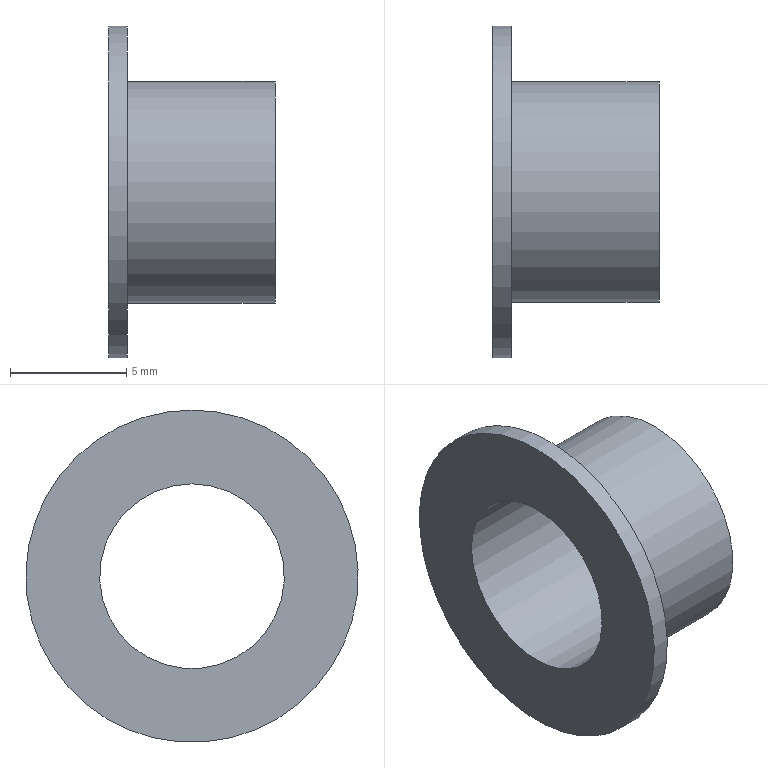Part | NX | features Igus GFI bushings(0.313 x 0.250) 2 | 1 solid | 6 faces | box 7.15 x 14.275 x 14.275 mm | volume 226.147 mm3 | plane 3 | cylinder 3 | commonest cylinder face diameters 7.938 x1 9.525 x1 14.275 x1
STEP:
#1=CARTESIAN_POINT('',(0.,0.,3.969));
#2=VERTEX_POINT('',#1);
#3=CARTESIAN_POINT('',(0.,0.,0.));
#4=DIRECTION('',(-1.,0.,0.));
#5=DIRECTION('',(0.,0.,1.));
#6=AXIS2_PLACEMENT_3D('',#3,#4,#5);
#7=CIRCLE('',#6,3.969);
#8=EDGE_CURVE('',#2,#2,#7,.T.);
#9=ORIENTED_EDGE('',*,*,#8,.F.);
#10=EDGE_LOOP('',(#9));
#11=FACE_BOUND('',#10,.T.);
#12=CARTESIAN_POINT('',(0.,0.,7.137));
#13=VERTEX_POINT('',#12);
#14=CARTESIAN_POINT('',(0.,0.,0.));
#15=DIRECTION('',(-1.,0.,0.));
#16=DIRECTION('',(0.,0.,1.));
#17=AXIS2_PLACEMENT_3D('',#14,#15,#16);
#18=CIRCLE('',#17,7.137);
#19=EDGE_CURVE('',#13,#13,#18,.T.);
#20=ORIENTED_EDGE('',*,*,#19,.T.);
#21=EDGE_LOOP('',(#20));
#22=FACE_BOUND('',#21,.T.);
#23=CARTESIAN_POINT('',(0.,3.969,0.));
#24=DIRECTION('',(1.,0.,0.));
#25=DIRECTION('',(0.,0.,-1.));
#26=AXIS2_PLACEMENT_3D('',#23,#24,#25);
#27=PLANE('',#26);
#28=ADVANCED_FACE('',(#11,#22),#27,.F.);
#29=ORIENTED_EDGE('',*,*,#19,.F.);
#30=EDGE_LOOP('',(#29));
#31=FACE_BOUND('',#30,.T.);
#32=CARTESIAN_POINT('',(0.7937,0.,7.137));
#33=VERTEX_POINT('',#32);
#34=CARTESIAN_POINT('',(0.7937,0.,0.));
#35=DIRECTION('',(-1.,0.,0.));
#36=DIRECTION('',(0.,0.,1.));
#37=AXIS2_PLACEMENT_3D('',#34,#35,#36);
#38=CIRCLE('',#37,7.137);
#39=EDGE_CURVE('',#33,#33,#38,.T.);
#40=ORIENTED_EDGE('',*,*,#39,.T.);
#41=EDGE_LOOP('',(#40));
#42=FACE_BOUND('',#41,.T.);
#43=CARTESIAN_POINT('',(0.,0.,0.));
#44=DIRECTION('',(-1.,0.,0.));
#45=DIRECTION('',(0.,0.,1.));
#46=AXIS2_PLACEMENT_3D('',#43,#44,#45);
#47=CYLINDRICAL_SURFACE('',#46,7.137);
#48=ADVANCED_FACE('',(#31,#42),#47,.T.);
#49=ORIENTED_EDGE('',*,*,#39,.F.);
#50=EDGE_LOOP('',(#49));
#51=FACE_BOUND('',#50,.T.);
#52=CARTESIAN_POINT('',(0.7937,0.,4.763));
#53=VERTEX_POINT('',#52);
#54=CARTESIAN_POINT('',(0.7937,0.,0.));
#55=DIRECTION('',(-1.,0.,0.));
#56=DIRECTION('',(0.,0.,1.));
#57=AXIS2_PLACEMENT_3D('',#54,#55,#56);
#58=CIRCLE('',#57,4.763);
#59=EDGE_CURVE('',#53,#53,#58,.T.);
#60=ORIENTED_EDGE('',*,*,#59,.T.);
#61=EDGE_LOOP('',(#60));
#62=FACE_BOUND('',#61,.T.);
#63=CARTESIAN_POINT('',(0.7937,4.763,0.));
#64=DIRECTION('',(-1.,0.,0.));
#65=DIRECTION('',(0.,0.,1.));
#66=AXIS2_PLACEMENT_3D('',#63,#64,#65);
#67=PLANE('',#66);
#68=ADVANCED_FACE('',(#51,#62),#67,.F.);
#69=ORIENTED_EDGE('',*,*,#59,.F.);
#70=EDGE_LOOP('',(#69));
#71=FACE_BOUND('',#70,.T.);
#72=CARTESIAN_POINT('',(7.15,0.,4.763));
#73=VERTEX_POINT('',#72);
#74=CARTESIAN_POINT('',(7.15,0.,0.));
#75=DIRECTION('',(-1.,0.,0.));
#76=DIRECTION('',(0.,0.,1.));
#77=AXIS2_PLACEMENT_3D('',#74,#75,#76);
#78=CIRCLE('',#77,4.763);
#79=EDGE_CURVE('',#73,#73,#78,.T.);
#80=ORIENTED_EDGE('',*,*,#79,.T.);
#81=EDGE_LOOP('',(#80));
#82=FACE_BOUND('',#81,.T.);
#83=CARTESIAN_POINT('',(0.,0.,0.));
#84=DIRECTION('',(-1.,0.,0.));
#85=DIRECTION('',(0.,0.,1.));
#86=AXIS2_PLACEMENT_3D('',#83,#84,#85);
#87=CYLINDRICAL_SURFACE('',#86,4.763);
#88=ADVANCED_FACE('',(#71,#82),#87,.T.);
#89=ORIENTED_EDGE('',*,*,#79,.F.);
#90=EDGE_LOOP('',(#89));
#91=FACE_BOUND('',#90,.T.);
#92=CARTESIAN_POINT('',(7.15,0.,3.969));
#93=VERTEX_POINT('',#92);
#94=CARTESIAN_POINT('',(7.15,0.,0.));
#95=DIRECTION('',(-1.,0.,0.));
#96=DIRECTION('',(0.,0.,1.));
#97=AXIS2_PLACEMENT_3D('',#94,#95,#96);
#98=CIRCLE('',#97,3.969);
#99=EDGE_CURVE('',#93,#93,#98,.T.);
#100=ORIENTED_EDGE('',*,*,#99,.T.);
#101=EDGE_LOOP('',(#100));
#102=FACE_BOUND('',#101,.T.);
#103=CARTESIAN_POINT('',(7.15,3.969,0.));
#104=DIRECTION('',(-1.,0.,0.));
#105=DIRECTION('',(0.,0.,1.));
#106=AXIS2_PLACEMENT_3D('',#103,#104,#105);
#107=PLANE('',#106);
#108=ADVANCED_FACE('',(#91,#102),#107,.F.);
#109=ORIENTED_EDGE('',*,*,#99,.F.);
#110=EDGE_LOOP('',(#109));
#111=FACE_BOUND('',#110,.T.);
#112=ORIENTED_EDGE('',*,*,#8,.T.);
#113=EDGE_LOOP('',(#112));
#114=FACE_BOUND('',#113,.T.);
#115=CARTESIAN_POINT('',(0.,0.,0.));
#116=DIRECTION('',(-1.,0.,0.));
#117=DIRECTION('',(0.,0.,1.));
#118=AXIS2_PLACEMENT_3D('',#115,#116,#117);
#119=CYLINDRICAL_SURFACE('',#118,3.969);
#120=ADVANCED_FACE('',(#111,#114),#119,.F.);
#121=CLOSED_SHELL('',(#28,#48,#68,#88,#108,#120));
#122=MANIFOLD_SOLID_BREP('',#121);
#123=(LENGTH_UNIT()NAMED_UNIT(*)SI_UNIT(.MILLI.,.METRE.));
#124=UNCERTAINTY_MEASURE_WITH_UNIT(LENGTH_MEASURE(0.00001),#123,'','');
#125=(NAMED_UNIT(*)PLANE_ANGLE_UNIT()SI_UNIT($,.RADIAN.));
#126=(NAMED_UNIT(*)SI_UNIT($,.STERADIAN.)SOLID_ANGLE_UNIT());
#127=(GEOMETRIC_REPRESENTATION_CONTEXT(3)GLOBAL_UNCERTAINTY_ASSIGNED_CONTEXT((#124))GLOBAL_UNIT_ASSIGNED_CONTEXT((#123,#125,#126))REPRESENTATION_CONTEXT('',''));
#128=ADVANCED_BREP_SHAPE_REPRESENTATION('',(#122),#127);